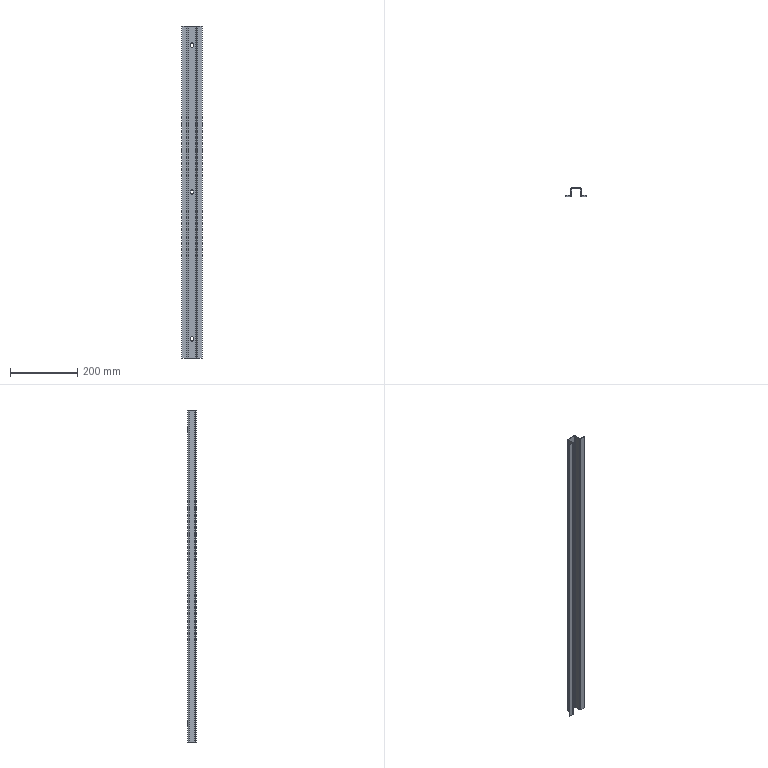Part | STEP file | SYL_0392D6J1SYL0380DJ100-399186 | 1 solid | 56 faces | box 60 x 25 x 984 mm | volume 197947 mm3 | plane 36 | cylinder 20 | commonest cylinder face diameters 7 x12 4 x4 8 x4
STEP:
#1=CARTESIAN_POINT('',(-3.5,23.,-431.5));
#2=VERTEX_POINT('',#1);
#3=CARTESIAN_POINT('',(-3.5,25.,-431.5));
#4=VERTEX_POINT('',#3);
#5=CARTESIAN_POINT('',(-3.5,25.,-431.5));
#6=DIRECTION('',(0.,1.,0.));
#7=VECTOR('',#6,1000.);
#8=LINE('',#5,#7);
#9=EDGE_CURVE('',#2,#4,#8,.T.);
#10=ORIENTED_EDGE('',*,*,#9,.F.);
#11=CARTESIAN_POINT('',(-3.5,23.,-438.5));
#12=VERTEX_POINT('',#11);
#13=CARTESIAN_POINT('',(-3.5,23.,-492.));
#14=DIRECTION('',(0.,0.,1.));
#15=VECTOR('',#14,1000.);
#16=LINE('',#13,#15);
#17=EDGE_CURVE('',#12,#2,#16,.T.);
#18=ORIENTED_EDGE('',*,*,#17,.F.);
#19=CARTESIAN_POINT('',(-3.5,25.,-438.5));
#20=VERTEX_POINT('',#19);
#21=CARTESIAN_POINT('',(-3.5,25.,-438.5));
#22=DIRECTION('',(0.,1.,0.));
#23=VECTOR('',#22,1000.);
#24=LINE('',#21,#23);
#25=EDGE_CURVE('',#12,#20,#24,.T.);
#26=ORIENTED_EDGE('',*,*,#25,.T.);
#27=CARTESIAN_POINT('',(-3.5,25.,-438.5));
#28=DIRECTION('',(0.,0.,1.));
#29=VECTOR('',#28,1000.);
#30=LINE('',#27,#29);
#31=EDGE_CURVE('',#20,#4,#30,.T.);
#32=ORIENTED_EDGE('',*,*,#31,.T.);
#33=EDGE_LOOP('',(#10,#18,#26,#32));
#34=FACE_OUTER_BOUND('',#33,.T.);
#35=CARTESIAN_POINT('',(-3.5,25.,-438.5));
#36=DIRECTION('',(1.,0.,0.));
#37=DIRECTION('',(0.,0.,1.));
#38=AXIS2_PLACEMENT_3D('',#35,#36,#37);
#39=PLANE('',#38);
#40=ADVANCED_FACE('',(#34),#39,.T.);
#41=ORIENTED_EDGE('',*,*,#25,.F.);
#42=CARTESIAN_POINT('',(0.,23.,-442.));
#43=VERTEX_POINT('',#42);
#44=CARTESIAN_POINT('',(0.,23.,-438.5));
#45=DIRECTION('',(0.,-1.,0.));
#46=DIRECTION('',(0.,0.,-1.));
#47=AXIS2_PLACEMENT_3D('',#44,#45,#46);
#48=CIRCLE('',#47,3.5);
#49=EDGE_CURVE('',#12,#43,#48,.T.);
#50=ORIENTED_EDGE('',*,*,#49,.T.);
#51=CARTESIAN_POINT('',(0.,25.,-442.));
#52=VERTEX_POINT('',#51);
#53=CARTESIAN_POINT('',(0.,25.,-442.));
#54=DIRECTION('',(0.,1.,0.));
#55=VECTOR('',#54,1000.);
#56=LINE('',#53,#55);
#57=EDGE_CURVE('',#43,#52,#56,.T.);
#58=ORIENTED_EDGE('',*,*,#57,.T.);
#59=CARTESIAN_POINT('',(0.,25.,-438.5));
#60=DIRECTION('',(0.,-1.,0.));
#61=DIRECTION('',(-1.,0.,0.));
#62=AXIS2_PLACEMENT_3D('',#59,#60,#61);
#63=CIRCLE('',#62,3.5);
#64=EDGE_CURVE('',#20,#52,#63,.T.);
#65=ORIENTED_EDGE('',*,*,#64,.F.);
#66=EDGE_LOOP('',(#41,#50,#58,#65));
#67=FACE_OUTER_BOUND('',#66,.T.);
#68=CARTESIAN_POINT('',(0.,25.,-438.5));
#69=DIRECTION('',(0.,-1.,0.));
#70=DIRECTION('',(0.,0.,-1.));
#71=AXIS2_PLACEMENT_3D('',#68,#69,#70);
#72=CYLINDRICAL_SURFACE('',#71,3.5);
#73=ADVANCED_FACE('',(#67),#72,.F.);
#74=ORIENTED_EDGE('',*,*,#57,.F.);
#75=CARTESIAN_POINT('',(3.5,23.,-438.5));
#76=VERTEX_POINT('',#75);
#77=CARTESIAN_POINT('',(0.,23.,-438.5));
#78=DIRECTION('',(0.,-1.,0.));
#79=DIRECTION('',(0.,0.,-1.));
#80=AXIS2_PLACEMENT_3D('',#77,#78,#79);
#81=CIRCLE('',#80,3.5);
#82=EDGE_CURVE('',#43,#76,#81,.T.);
#83=ORIENTED_EDGE('',*,*,#82,.T.);
#84=CARTESIAN_POINT('',(3.5,25.,-438.5));
#85=VERTEX_POINT('',#84);
#86=CARTESIAN_POINT('',(3.5,25.,-438.5));
#87=DIRECTION('',(0.,1.,0.));
#88=VECTOR('',#87,1000.);
#89=LINE('',#86,#88);
#90=EDGE_CURVE('',#76,#85,#89,.T.);
#91=ORIENTED_EDGE('',*,*,#90,.T.);
#92=CARTESIAN_POINT('',(0.,25.,-438.5));
#93=DIRECTION('',(0.,-1.,0.));
#94=DIRECTION('',(0.,0.,-1.));
#95=AXIS2_PLACEMENT_3D('',#92,#93,#94);
#96=CIRCLE('',#95,3.5);
#97=EDGE_CURVE('',#52,#85,#96,.T.);
#98=ORIENTED_EDGE('',*,*,#97,.F.);
#99=EDGE_LOOP('',(#74,#83,#91,#98));
#100=FACE_OUTER_BOUND('',#99,.T.);
#101=CARTESIAN_POINT('',(0.,25.,-438.5));
#102=DIRECTION('',(0.,-1.,0.));
#103=DIRECTION('',(0.,0.,-1.));
#104=AXIS2_PLACEMENT_3D('',#101,#102,#103);
#105=CYLINDRICAL_SURFACE('',#104,3.5);
#106=ADVANCED_FACE('',(#100),#105,.F.);
#107=ORIENTED_EDGE('',*,*,#90,.F.);
#108=CARTESIAN_POINT('',(3.5,23.,-431.5));
#109=VERTEX_POINT('',#108);
#110=CARTESIAN_POINT('',(3.5,23.,-492.));
#111=DIRECTION('',(0.,0.,-1.));
#112=VECTOR('',#111,1000.);
#113=LINE('',#110,#112);
#114=EDGE_CURVE('',#109,#76,#113,.T.);
#115=ORIENTED_EDGE('',*,*,#114,.F.);
#116=CARTESIAN_POINT('',(3.5,25.,-431.5));
#117=VERTEX_POINT('',#116);
#118=CARTESIAN_POINT('',(3.5,25.,-431.5));
#119=DIRECTION('',(0.,1.,0.));
#120=VECTOR('',#119,1000.);
#121=LINE('',#118,#120);
#122=EDGE_CURVE('',#109,#117,#121,.T.);
#123=ORIENTED_EDGE('',*,*,#122,.T.);
#124=CARTESIAN_POINT('',(3.5,25.,-431.5));
#125=DIRECTION('',(0.,0.,-1.));
#126=VECTOR('',#125,1000.);
#127=LINE('',#124,#126);
#128=EDGE_CURVE('',#117,#85,#127,.T.);
#129=ORIENTED_EDGE('',*,*,#128,.T.);
#130=EDGE_LOOP('',(#107,#115,#123,#129));
#131=FACE_OUTER_BOUND('',#130,.T.);
#132=CARTESIAN_POINT('',(3.5,25.,-431.5));
#133=DIRECTION('',(-1.,0.,0.));
#134=DIRECTION('',(0.,0.,-1.));
#135=AXIS2_PLACEMENT_3D('',#132,#133,#134);
#136=PLANE('',#135);
#137=ADVANCED_FACE('',(#131),#136,.T.);
#138=ORIENTED_EDGE('',*,*,#122,.F.);
#139=CARTESIAN_POINT('',(0.,23.,-428.));
#140=VERTEX_POINT('',#139);
#141=CARTESIAN_POINT('',(0.,23.,-431.5));
#142=DIRECTION('',(0.,-1.,0.));
#143=DIRECTION('',(0.,0.,-1.));
#144=AXIS2_PLACEMENT_3D('',#141,#142,#143);
#145=CIRCLE('',#144,3.5);
#146=EDGE_CURVE('',#109,#140,#145,.T.);
#147=ORIENTED_EDGE('',*,*,#146,.T.);
#148=CARTESIAN_POINT('',(0.,25.,-428.));
#149=VERTEX_POINT('',#148);
#150=CARTESIAN_POINT('',(0.,25.,-428.));
#151=DIRECTION('',(0.,1.,0.));
#152=VECTOR('',#151,1000.);
#153=LINE('',#150,#152);
#154=EDGE_CURVE('',#140,#149,#153,.T.);
#155=ORIENTED_EDGE('',*,*,#154,.T.);
#156=CARTESIAN_POINT('',(0.,25.,-431.5));
#157=DIRECTION('',(0.,-1.,0.));
#158=DIRECTION('',(1.,0.,0.));
#159=AXIS2_PLACEMENT_3D('',#156,#157,#158);
#160=CIRCLE('',#159,3.5);
#161=EDGE_CURVE('',#117,#149,#160,.T.);
#162=ORIENTED_EDGE('',*,*,#161,.F.);
#163=EDGE_LOOP('',(#138,#147,#155,#162));
#164=FACE_OUTER_BOUND('',#163,.T.);
#165=CARTESIAN_POINT('',(0.,25.,-431.5));
#166=DIRECTION('',(0.,-1.,0.));
#167=DIRECTION('',(0.,0.,-1.));
#168=AXIS2_PLACEMENT_3D('',#165,#166,#167);
#169=CYLINDRICAL_SURFACE('',#168,3.5);
#170=ADVANCED_FACE('',(#164),#169,.F.);
#171=CARTESIAN_POINT('',(-3.5,23.,3.5));
#172=VERTEX_POINT('',#171);
#173=CARTESIAN_POINT('',(-3.5,25.,3.5));
#174=VERTEX_POINT('',#173);
#175=CARTESIAN_POINT('',(-3.5,25.,3.5));
#176=DIRECTION('',(0.,1.,0.));
#177=VECTOR('',#176,1000.);
#178=LINE('',#175,#177);
#179=EDGE_CURVE('',#172,#174,#178,.T.);
#180=ORIENTED_EDGE('',*,*,#179,.F.);
#181=CARTESIAN_POINT('',(-3.5,23.,-3.5));
#182=VERTEX_POINT('',#181);
#183=CARTESIAN_POINT('',(-3.5,23.,-492.));
#184=DIRECTION('',(0.,0.,1.));
#185=VECTOR('',#184,1000.);
#186=LINE('',#183,#185);
#187=EDGE_CURVE('',#182,#172,#186,.T.);
#188=ORIENTED_EDGE('',*,*,#187,.F.);
#189=CARTESIAN_POINT('',(-3.5,25.,-3.5));
#190=VERTEX_POINT('',#189);
#191=CARTESIAN_POINT('',(-3.5,25.,-3.5));
#192=DIRECTION('',(0.,1.,0.));
#193=VECTOR('',#192,1000.);
#194=LINE('',#191,#193);
#195=EDGE_CURVE('',#182,#190,#194,.T.);
#196=ORIENTED_EDGE('',*,*,#195,.T.);
#197=CARTESIAN_POINT('',(-3.5,25.,-3.5));
#198=DIRECTION('',(0.,0.,1.));
#199=VECTOR('',#198,1000.);
#200=LINE('',#197,#199);
#201=EDGE_CURVE('',#190,#174,#200,.T.);
#202=ORIENTED_EDGE('',*,*,#201,.T.);
#203=EDGE_LOOP('',(#180,#188,#196,#202));
#204=FACE_OUTER_BOUND('',#203,.T.);
#205=CARTESIAN_POINT('',(-3.5,25.,-3.5));
#206=DIRECTION('',(1.,0.,0.));
#207=DIRECTION('',(0.,0.,1.));
#208=AXIS2_PLACEMENT_3D('',#205,#206,#207);
#209=PLANE('',#208);
#210=ADVANCED_FACE('',(#204),#209,.T.);
#211=ORIENTED_EDGE('',*,*,#195,.F.);
#212=CARTESIAN_POINT('',(0.,23.,-7.));
#213=VERTEX_POINT('',#212);
#214=CARTESIAN_POINT('',(0.,23.,-3.5));
#215=DIRECTION('',(0.,-1.,0.));
#216=DIRECTION('',(0.,0.,-1.));
#217=AXIS2_PLACEMENT_3D('',#214,#215,#216);
#218=CIRCLE('',#217,3.5);
#219=EDGE_CURVE('',#182,#213,#218,.T.);
#220=ORIENTED_EDGE('',*,*,#219,.T.);
#221=CARTESIAN_POINT('',(0.,25.,-7.));
#222=VERTEX_POINT('',#221);
#223=CARTESIAN_POINT('',(0.,25.,-7.));
#224=DIRECTION('',(0.,1.,0.));
#225=VECTOR('',#224,1000.);
#226=LINE('',#223,#225);
#227=EDGE_CURVE('',#213,#222,#226,.T.);
#228=ORIENTED_EDGE('',*,*,#227,.T.);
#229=CARTESIAN_POINT('',(0.,25.,-3.5));
#230=DIRECTION('',(0.,-1.,0.));
#231=DIRECTION('',(-1.,0.,0.));
#232=AXIS2_PLACEMENT_3D('',#229,#230,#231);
#233=CIRCLE('',#232,3.5);
#234=EDGE_CURVE('',#190,#222,#233,.T.);
#235=ORIENTED_EDGE('',*,*,#234,.F.);
#236=EDGE_LOOP('',(#211,#220,#228,#235));
#237=FACE_OUTER_BOUND('',#236,.T.);
#238=CARTESIAN_POINT('',(0.,25.,-3.5));
#239=DIRECTION('',(0.,-1.,0.));
#240=DIRECTION('',(0.,0.,-1.));
#241=AXIS2_PLACEMENT_3D('',#238,#239,#240);
#242=CYLINDRICAL_SURFACE('',#241,3.5);
#243=ADVANCED_FACE('',(#237),#242,.F.);
#244=ORIENTED_EDGE('',*,*,#227,.F.);
#245=CARTESIAN_POINT('',(3.5,23.,-3.5));
#246=VERTEX_POINT('',#245);
#247=CARTESIAN_POINT('',(0.,23.,-3.5));
#248=DIRECTION('',(0.,-1.,0.));
#249=DIRECTION('',(0.,0.,-1.));
#250=AXIS2_PLACEMENT_3D('',#247,#248,#249);
#251=CIRCLE('',#250,3.5);
#252=EDGE_CURVE('',#213,#246,#251,.T.);
#253=ORIENTED_EDGE('',*,*,#252,.T.);
#254=CARTESIAN_POINT('',(3.5,25.,-3.5));
#255=VERTEX_POINT('',#254);
#256=CARTESIAN_POINT('',(3.5,25.,-3.5));
#257=DIRECTION('',(0.,1.,0.));
#258=VECTOR('',#257,1000.);
#259=LINE('',#256,#258);
#260=EDGE_CURVE('',#246,#255,#259,.T.);
#261=ORIENTED_EDGE('',*,*,#260,.T.);
#262=CARTESIAN_POINT('',(0.,25.,-3.5));
#263=DIRECTION('',(0.,-1.,0.));
#264=DIRECTION('',(0.,0.,-1.));
#265=AXIS2_PLACEMENT_3D('',#262,#263,#264);
#266=CIRCLE('',#265,3.5);
#267=EDGE_CURVE('',#222,#255,#266,.T.);
#268=ORIENTED_EDGE('',*,*,#267,.F.);
#269=EDGE_LOOP('',(#244,#253,#261,#268));
#270=FACE_OUTER_BOUND('',#269,.T.);
#271=CARTESIAN_POINT('',(0.,25.,-3.5));
#272=DIRECTION('',(0.,-1.,0.));
#273=DIRECTION('',(0.,0.,-1.));
#274=AXIS2_PLACEMENT_3D('',#271,#272,#273);
#275=CYLINDRICAL_SURFACE('',#274,3.5);
#276=ADVANCED_FACE('',(#270),#275,.F.);
#277=ORIENTED_EDGE('',*,*,#260,.F.);
#278=CARTESIAN_POINT('',(3.5,23.,3.5));
#279=VERTEX_POINT('',#278);
#280=CARTESIAN_POINT('',(3.5,23.,-492.));
#281=DIRECTION('',(0.,0.,-1.));
#282=VECTOR('',#281,1000.);
#283=LINE('',#280,#282);
#284=EDGE_CURVE('',#279,#246,#283,.T.);
#285=ORIENTED_EDGE('',*,*,#284,.F.);
#286=CARTESIAN_POINT('',(3.5,25.,3.5));
#287=VERTEX_POINT('',#286);
#288=CARTESIAN_POINT('',(3.5,25.,3.5));
#289=DIRECTION('',(0.,1.,0.));
#290=VECTOR('',#289,1000.);
#291=LINE('',#288,#290);
#292=EDGE_CURVE('',#279,#287,#291,.T.);
#293=ORIENTED_EDGE('',*,*,#292,.T.);
#294=CARTESIAN_POINT('',(3.5,25.,3.5));
#295=DIRECTION('',(0.,0.,-1.));
#296=VECTOR('',#295,1000.);
#297=LINE('',#294,#296);
#298=EDGE_CURVE('',#287,#255,#297,.T.);
#299=ORIENTED_EDGE('',*,*,#298,.T.);
#300=EDGE_LOOP('',(#277,#285,#293,#299));
#301=FACE_OUTER_BOUND('',#300,.T.);
#302=CARTESIAN_POINT('',(3.5,25.,3.5));
#303=DIRECTION('',(-1.,0.,0.));
#304=DIRECTION('',(0.,0.,-1.));
#305=AXIS2_PLACEMENT_3D('',#302,#303,#304);
#306=PLANE('',#305);
#307=ADVANCED_FACE('',(#301),#306,.T.);
#308=ORIENTED_EDGE('',*,*,#292,.F.);
#309=CARTESIAN_POINT('',(0.,23.,7.));
#310=VERTEX_POINT('',#309);
#311=CARTESIAN_POINT('',(0.,23.,3.5));
#312=DIRECTION('',(0.,-1.,0.));
#313=DIRECTION('',(0.,0.,-1.));
#314=AXIS2_PLACEMENT_3D('',#311,#312,#313);
#315=CIRCLE('',#314,3.5);
#316=EDGE_CURVE('',#279,#310,#315,.T.);
#317=ORIENTED_EDGE('',*,*,#316,.T.);
#318=CARTESIAN_POINT('',(0.,25.,7.));
#319=VERTEX_POINT('',#318);
#320=CARTESIAN_POINT('',(0.,25.,7.));
#321=DIRECTION('',(0.,1.,0.));
#322=VECTOR('',#321,1000.);
#323=LINE('',#320,#322);
#324=EDGE_CURVE('',#310,#319,#323,.T.);
#325=ORIENTED_EDGE('',*,*,#324,.T.);
#326=CARTESIAN_POINT('',(0.,25.,3.5));
#327=DIRECTION('',(0.,-1.,0.));
#328=DIRECTION('',(1.,0.,0.));
#329=AXIS2_PLACEMENT_3D('',#326,#327,#328);
#330=CIRCLE('',#329,3.5);
#331=EDGE_CURVE('',#287,#319,#330,.T.);
#332=ORIENTED_EDGE('',*,*,#331,.F.);
#333=EDGE_LOOP('',(#308,#317,#325,#332));
#334=FACE_OUTER_BOUND('',#333,.T.);
#335=CARTESIAN_POINT('',(0.,25.,3.5));
#336=DIRECTION('',(0.,-1.,0.));
#337=DIRECTION('',(0.,0.,-1.));
#338=AXIS2_PLACEMENT_3D('',#335,#336,#337);
#339=CYLINDRICAL_SURFACE('',#338,3.5);
#340=ADVANCED_FACE('',(#334),#339,.F.);
#341=CARTESIAN_POINT('',(-3.5,23.,438.5));
#342=VERTEX_POINT('',#341);
#343=CARTESIAN_POINT('',(-3.5,25.,438.5));
#344=VERTEX_POINT('',#343);
#345=CARTESIAN_POINT('',(-3.5,25.,438.5));
#346=DIRECTION('',(0.,1.,0.));
#347=VECTOR('',#346,1000.);
#348=LINE('',#345,#347);
#349=EDGE_CURVE('',#342,#344,#348,.T.);
#350=ORIENTED_EDGE('',*,*,#349,.F.);
#351=CARTESIAN_POINT('',(-3.5,23.,431.5));
#352=VERTEX_POINT('',#351);
#353=CARTESIAN_POINT('',(-3.5,23.,-492.));
#354=DIRECTION('',(0.,0.,1.));
#355=VECTOR('',#354,1000.);
#356=LINE('',#353,#355);
#357=EDGE_CURVE('',#352,#342,#356,.T.);
#358=ORIENTED_EDGE('',*,*,#357,.F.);
#359=CARTESIAN_POINT('',(-3.5,25.,431.5));
#360=VERTEX_POINT('',#359);
#361=CARTESIAN_POINT('',(-3.5,25.,431.5));
#362=DIRECTION('',(0.,1.,0.));
#363=VECTOR('',#362,1000.);
#364=LINE('',#361,#363);
#365=EDGE_CURVE('',#352,#360,#364,.T.);
#366=ORIENTED_EDGE('',*,*,#365,.T.);
#367=CARTESIAN_POINT('',(-3.5,25.,431.5));
#368=DIRECTION('',(0.,0.,1.));
#369=VECTOR('',#368,1000.);
#370=LINE('',#367,#369);
#371=EDGE_CURVE('',#360,#344,#370,.T.);
#372=ORIENTED_EDGE('',*,*,#371,.T.);
#373=EDGE_LOOP('',(#350,#358,#366,#372));
#374=FACE_OUTER_BOUND('',#373,.T.);
#375=CARTESIAN_POINT('',(-3.5,25.,431.5));
#376=DIRECTION('',(1.,0.,0.));
#377=DIRECTION('',(0.,0.,1.));
#378=AXIS2_PLACEMENT_3D('',#375,#376,#377);
#379=PLANE('',#378);
#380=ADVANCED_FACE('',(#374),#379,.T.);
#381=ORIENTED_EDGE('',*,*,#365,.F.);
#382=CARTESIAN_POINT('',(0.,23.,428.));
#383=VERTEX_POINT('',#382);
#384=CARTESIAN_POINT('',(0.,23.,431.5));
#385=DIRECTION('',(0.,-1.,0.));
#386=DIRECTION('',(0.,0.,-1.));
#387=AXIS2_PLACEMENT_3D('',#384,#385,#386);
#388=CIRCLE('',#387,3.5);
#389=EDGE_CURVE('',#352,#383,#388,.T.);
#390=ORIENTED_EDGE('',*,*,#389,.T.);
#391=CARTESIAN_POINT('',(0.,25.,428.));
#392=VERTEX_POINT('',#391);
#393=CARTESIAN_POINT('',(0.,25.,428.));
#394=DIRECTION('',(0.,1.,0.));
#395=VECTOR('',#394,1000.);
#396=LINE('',#393,#395);
#397=EDGE_CURVE('',#383,#392,#396,.T.);
#398=ORIENTED_EDGE('',*,*,#397,.T.);
#399=CARTESIAN_POINT('',(0.,25.,431.5));
#400=DIRECTION('',(0.,-1.,0.));
#401=DIRECTION('',(-1.,0.,0.));
#402=AXIS2_PLACEMENT_3D('',#399,#400,#401);
#403=CIRCLE('',#402,3.5);
#404=EDGE_CURVE('',#360,#392,#403,.T.);
#405=ORIENTED_EDGE('',*,*,#404,.F.);
#406=EDGE_LOOP('',(#381,#390,#398,#405));
#407=FACE_OUTER_BOUND('',#406,.T.);
#408=CARTESIAN_POINT('',(0.,25.,431.5));
#409=DIRECTION('',(0.,-1.,0.));
#410=DIRECTION('',(0.,0.,-1.));
#411=AXIS2_PLACEMENT_3D('',#408,#409,#410);
#412=CYLINDRICAL_SURFACE('',#411,3.5);
#413=ADVANCED_FACE('',(#407),#412,.F.);
#414=ORIENTED_EDGE('',*,*,#397,.F.);
#415=CARTESIAN_POINT('',(3.5,23.,431.5));
#416=VERTEX_POINT('',#415);
#417=CARTESIAN_POINT('',(0.,23.,431.5));
#418=DIRECTION('',(0.,-1.,0.));
#419=DIRECTION('',(0.,0.,-1.));
#420=AXIS2_PLACEMENT_3D('',#417,#418,#419);
#421=CIRCLE('',#420,3.5);
#422=EDGE_CURVE('',#383,#416,#421,.T.);
#423=ORIENTED_EDGE('',*,*,#422,.T.);
#424=CARTESIAN_POINT('',(3.5,25.,431.5));
#425=VERTEX_POINT('',#424);
#426=CARTESIAN_POINT('',(3.5,25.,431.5));
#427=DIRECTION('',(0.,1.,0.));
#428=VECTOR('',#427,1000.);
#429=LINE('',#426,#428);
#430=EDGE_CURVE('',#416,#425,#429,.T.);
#431=ORIENTED_EDGE('',*,*,#430,.T.);
#432=CARTESIAN_POINT('',(0.,25.,431.5));
#433=DIRECTION('',(0.,-1.,0.));
#434=DIRECTION('',(0.,0.,-1.));
#435=AXIS2_PLACEMENT_3D('',#432,#433,#434);
#436=CIRCLE('',#435,3.5);
#437=EDGE_CURVE('',#392,#425,#436,.T.);
#438=ORIENTED_EDGE('',*,*,#437,.F.);
#439=EDGE_LOOP('',(#414,#423,#431,#438));
#440=FACE_OUTER_BOUND('',#439,.T.);
#441=CARTESIAN_POINT('',(0.,25.,431.5));
#442=DIRECTION('',(0.,-1.,0.));
#443=DIRECTION('',(0.,0.,-1.));
#444=AXIS2_PLACEMENT_3D('',#441,#442,#443);
#445=CYLINDRICAL_SURFACE('',#444,3.5);
#446=ADVANCED_FACE('',(#440),#445,.F.);
#447=ORIENTED_EDGE('',*,*,#430,.F.);
#448=CARTESIAN_POINT('',(3.5,23.,438.5));
#449=VERTEX_POINT('',#448);
#450=CARTESIAN_POINT('',(3.5,23.,-492.));
#451=DIRECTION('',(0.,0.,-1.));
#452=VECTOR('',#451,1000.);
#453=LINE('',#450,#452);
#454=EDGE_CURVE('',#449,#416,#453,.T.);
#455=ORIENTED_EDGE('',*,*,#454,.F.);
#456=CARTESIAN_POINT('',(3.5,25.,438.5));
#457=VERTEX_POINT('',#456);
#458=CARTESIAN_POINT('',(3.5,25.,438.5));
#459=DIRECTION('',(0.,1.,0.));
#460=VECTOR('',#459,1000.);
#461=LINE('',#458,#460);
#462=EDGE_CURVE('',#449,#457,#461,.T.);
#463=ORIENTED_EDGE('',*,*,#462,.T.);
#464=CARTESIAN_POINT('',(3.5,25.,438.5));
#465=DIRECTION('',(0.,0.,-1.));
#466=VECTOR('',#465,1000.);
#467=LINE('',#464,#466);
#468=EDGE_CURVE('',#457,#425,#467,.T.);
#469=ORIENTED_EDGE('',*,*,#468,.T.);
#470=EDGE_LOOP('',(#447,#455,#463,#469));
#471=FACE_OUTER_BOUND('',#470,.T.);
#472=CARTESIAN_POINT('',(3.5,25.,438.5));
#473=DIRECTION('',(-1.,0.,0.));
#474=DIRECTION('',(0.,0.,-1.));
#475=AXIS2_PLACEMENT_3D('',#472,#473,#474);
#476=PLANE('',#475);
#477=ADVANCED_FACE('',(#471),#476,.T.);
#478=ORIENTED_EDGE('',*,*,#462,.F.);
#479=CARTESIAN_POINT('',(0.,23.,442.));
#480=VERTEX_POINT('',#479);
#481=CARTESIAN_POINT('',(0.,23.,438.5));
#482=DIRECTION('',(0.,-1.,0.));
#483=DIRECTION('',(0.,0.,-1.));
#484=AXIS2_PLACEMENT_3D('',#481,#482,#483);
#485=CIRCLE('',#484,3.5);
#486=EDGE_CURVE('',#449,#480,#485,.T.);
#487=ORIENTED_EDGE('',*,*,#486,.T.);
#488=CARTESIAN_POINT('',(0.,25.,442.));
#489=VERTEX_POINT('',#488);
#490=CARTESIAN_POINT('',(0.,25.,442.));
#491=DIRECTION('',(0.,1.,0.));
#492=VECTOR('',#491,1000.);
#493=LINE('',#490,#492);
#494=EDGE_CURVE('',#480,#489,#493,.T.);
#495=ORIENTED_EDGE('',*,*,#494,.T.);
#496=CARTESIAN_POINT('',(0.,25.,438.5));
#497=DIRECTION('',(0.,-1.,0.));
#498=DIRECTION('',(1.,0.,0.));
#499=AXIS2_PLACEMENT_3D('',#496,#497,#498);
#500=CIRCLE('',#499,3.5);
#501=EDGE_CURVE('',#457,#489,#500,.T.);
#502=ORIENTED_EDGE('',*,*,#501,.F.);
#503=EDGE_LOOP('',(#478,#487,#495,#502));
#504=FACE_OUTER_BOUND('',#503,.T.);
#505=CARTESIAN_POINT('',(0.,25.,438.5));
#506=DIRECTION('',(0.,-1.,0.));
#507=DIRECTION('',(0.,0.,-1.));
#508=AXIS2_PLACEMENT_3D('',#505,#506,#507);
#509=CYLINDRICAL_SURFACE('',#508,3.5);
#510=ADVANCED_FACE('',(#504),#509,.F.);
#511=CARTESIAN_POINT('',(-30.,0.,-492.));
#512=VERTEX_POINT('',#511);
#513=CARTESIAN_POINT('',(-30.,2.,-492.));
#514=VERTEX_POINT('',#513);
#515=CARTESIAN_POINT('',(-30.,2.,-492.));
#516=DIRECTION('',(0.,1.,0.));
#517=VECTOR('',#516,1000.);
#518=LINE('',#515,#517);
#519=EDGE_CURVE('',#512,#514,#518,.T.);
#520=ORIENTED_EDGE('',*,*,#519,.F.);
#521=CARTESIAN_POINT('',(-30.,0.,492.));
#522=VERTEX_POINT('',#521);
#523=CARTESIAN_POINT('',(-30.,0.,-492.));
#524=DIRECTION('',(0.,0.,-1.));
#525=VECTOR('',#524,1000.);
#526=LINE('',#523,#525);
#527=EDGE_CURVE('',#522,#512,#526,.T.);
#528=ORIENTED_EDGE('',*,*,#527,.F.);
#529=CARTESIAN_POINT('',(-30.,2.,492.));
#530=VERTEX_POINT('',#529);
#531=CARTESIAN_POINT('',(-30.,2.,492.));
#532=DIRECTION('',(0.,1.,0.));
#533=VECTOR('',#532,1000.);
#534=LINE('',#531,#533);
#535=EDGE_CURVE('',#522,#530,#534,.T.);
#536=ORIENTED_EDGE('',*,*,#535,.T.);
#537=CARTESIAN_POINT('',(-30.,2.,492.));
#538=DIRECTION('',(0.,0.,-1.));
#539=VECTOR('',#538,1000.);
#540=LINE('',#537,#539);
#541=EDGE_CURVE('',#530,#514,#540,.T.);
#542=ORIENTED_EDGE('',*,*,#541,.T.);
#543=EDGE_LOOP('',(#520,#528,#536,#542));
#544=FACE_OUTER_BOUND('',#543,.T.);
#545=CARTESIAN_POINT('',(-30.,2.,492.));
#546=DIRECTION('',(-1.,0.,0.));
#547=DIRECTION('',(0.,0.,-1.));
#548=AXIS2_PLACEMENT_3D('',#545,#546,#547);
#549=PLANE('',#548);
#550=ADVANCED_FACE('',(#544),#549,.T.);
#551=ORIENTED_EDGE('',*,*,#535,.F.);
#552=CARTESIAN_POINT('',(-17.,0.,492.));
#553=VERTEX_POINT('',#552);
#554=CARTESIAN_POINT('',(-30.,0.,492.));
#555=DIRECTION('',(-1.,0.,0.));
#556=VECTOR('',#555,1000.);
#557=LINE('',#554,#556);
#558=EDGE_CURVE('',#553,#522,#557,.T.);
#559=ORIENTED_EDGE('',*,*,#558,.F.);
#560=CARTESIAN_POINT('',(-17.,2.,492.));
#561=VERTEX_POINT('',#560);
#562=CARTESIAN_POINT('',(-17.,2.,492.));
#563=DIRECTION('',(0.,1.,0.));
#564=VECTOR('',#563,1000.);
#565=LINE('',#562,#564);
#566=EDGE_CURVE('',#553,#561,#565,.T.);
#567=ORIENTED_EDGE('',*,*,#566,.T.);
#568=CARTESIAN_POINT('',(-17.,2.,492.));
#569=DIRECTION('',(-1.,0.,0.));
#570=VECTOR('',#569,1000.);
#571=LINE('',#568,#570);
#572=EDGE_CURVE('',#561,#530,#571,.T.);
#573=ORIENTED_EDGE('',*,*,#572,.T.);
#574=EDGE_LOOP('',(#551,#559,#567,#573));
#575=FACE_OUTER_BOUND('',#574,.T.);
#576=CARTESIAN_POINT('',(-17.,2.,492.));
#577=DIRECTION('',(0.,0.,1.));
#578=DIRECTION('',(-1.,0.,0.));
#579=AXIS2_PLACEMENT_3D('',#576,#577,#578);
#580=PLANE('',#579);
#581=ADVANCED_FACE('',(#575),#580,.T.);
#582=ORIENTED_EDGE('',*,*,#566,.F.);
#583=CARTESIAN_POINT('',(-13.,4.,492.));
#584=VERTEX_POINT('',#583);
#585=CARTESIAN_POINT('',(-17.,4.,492.));
#586=DIRECTION('',(0.,0.,-1.));
#587=DIRECTION('',(1.,0.,0.));
#588=AXIS2_PLACEMENT_3D('',#585,#586,#587);
#589=CIRCLE('',#588,4.);
#590=EDGE_CURVE('',#584,#553,#589,.T.);
#591=ORIENTED_EDGE('',*,*,#590,.F.);
#592=CARTESIAN_POINT('',(-15.,4.,492.));
#593=VERTEX_POINT('',#592);
#594=CARTESIAN_POINT('',(-15.,4.,492.));
#595=DIRECTION('',(-1.,0.,0.));
#596=VECTOR('',#595,1000.);
#597=LINE('',#594,#596);
#598=EDGE_CURVE('',#584,#593,#597,.T.);
#599=ORIENTED_EDGE('',*,*,#598,.T.);
#600=CARTESIAN_POINT('',(-17.,4.,492.));
#601=DIRECTION('',(0.,0.,-1.));
#602=DIRECTION('',(1.,0.,0.));
#603=AXIS2_PLACEMENT_3D('',#600,#601,#602);
#604=CIRCLE('',#603,2.);
#605=EDGE_CURVE('',#593,#561,#604,.T.);
#606=ORIENTED_EDGE('',*,*,#605,.T.);
#607=EDGE_LOOP('',(#582,#591,#599,#606));
#608=FACE_OUTER_BOUND('',#607,.T.);
#609=CARTESIAN_POINT('',(-17.,4.,492.));
#610=DIRECTION('',(0.,0.,1.));
#611=DIRECTION('',(1.,0.,0.));
#612=AXIS2_PLACEMENT_3D('',#609,#610,#611);
#613=PLANE('',#612);
#614=ADVANCED_FACE('',(#608),#613,.T.);
#615=ORIENTED_EDGE('',*,*,#598,.F.);
#616=CARTESIAN_POINT('',(-13.,21.,492.));
#617=VERTEX_POINT('',#616);
#618=CARTESIAN_POINT('',(-13.,4.,492.));
#619=DIRECTION('',(0.,-1.,0.));
#620=VECTOR('',#619,1000.);
#621=LINE('',#618,#620);
#622=EDGE_CURVE('',#617,#584,#621,.T.);
#623=ORIENTED_EDGE('',*,*,#622,.F.);
#624=CARTESIAN_POINT('',(-15.,21.,492.));
#625=VERTEX_POINT('',#624);
#626=CARTESIAN_POINT('',(-15.,21.,492.));
#627=DIRECTION('',(-1.,0.,0.));
#628=VECTOR('',#627,1000.);
#629=LINE('',#626,#628);
#630=EDGE_CURVE('',#617,#625,#629,.T.);
#631=ORIENTED_EDGE('',*,*,#630,.T.);
#632=CARTESIAN_POINT('',(-15.,21.,492.));
#633=DIRECTION('',(0.,-1.,0.));
#634=VECTOR('',#633,1000.);
#635=LINE('',#632,#634);
#636=EDGE_CURVE('',#625,#593,#635,.T.);
#637=ORIENTED_EDGE('',*,*,#636,.T.);
#638=EDGE_LOOP('',(#615,#623,#631,#637));
#639=FACE_OUTER_BOUND('',#638,.T.);
#640=CARTESIAN_POINT('',(-15.,21.,492.));
#641=DIRECTION('',(0.,0.,1.));
#642=DIRECTION('',(0.,-1.,0.));
#643=AXIS2_PLACEMENT_3D('',#640,#641,#642);
#644=PLANE('',#643);
#645=ADVANCED_FACE('',(#639),#644,.T.);
#646=ORIENTED_EDGE('',*,*,#630,.F.);
#647=CARTESIAN_POINT('',(-11.,23.,492.));
#648=VERTEX_POINT('',#647);
#649=CARTESIAN_POINT('',(-11.,21.,492.));
#650=DIRECTION('',(0.,0.,1.));
#651=DIRECTION('',(1.,0.,0.));
#652=AXIS2_PLACEMENT_3D('',#649,#650,#651);
#653=CIRCLE('',#652,2.);
#654=EDGE_CURVE('',#648,#617,#653,.T.);
#655=ORIENTED_EDGE('',*,*,#654,.F.);
#656=CARTESIAN_POINT('',(-11.,25.,492.));
#657=VERTEX_POINT('',#656);
#658=CARTESIAN_POINT('',(-11.,25.,492.));
#659=DIRECTION('',(0.,1.,0.));
#660=VECTOR('',#659,1000.);
#661=LINE('',#658,#660);
#662=EDGE_CURVE('',#648,#657,#661,.T.);
#663=ORIENTED_EDGE('',*,*,#662,.T.);
#664=CARTESIAN_POINT('',(-11.,21.,492.));
#665=DIRECTION('',(0.,0.,1.));
#666=DIRECTION('',(0.,1.,0.));
#667=AXIS2_PLACEMENT_3D('',#664,#665,#666);
#668=CIRCLE('',#667,4.);
#669=EDGE_CURVE('',#657,#625,#668,.T.);
#670=ORIENTED_EDGE('',*,*,#669,.T.);
#671=EDGE_LOOP('',(#646,#655,#663,#670));
#672=FACE_OUTER_BOUND('',#671,.T.);
#673=CARTESIAN_POINT('',(-11.,21.,492.));
#674=DIRECTION('',(0.,0.,-1.));
#675=DIRECTION('',(-1.,0.,0.));
#676=AXIS2_PLACEMENT_3D('',#673,#674,#675);
#677=PLANE('',#676);
#678=ADVANCED_FACE('',(#672),#677,.F.);
#679=ORIENTED_EDGE('',*,*,#662,.F.);
#680=CARTESIAN_POINT('',(11.,23.,492.));
#681=VERTEX_POINT('',#680);
#682=CARTESIAN_POINT('',(-11.,23.,492.));
#683=DIRECTION('',(-1.,0.,0.));
#684=VECTOR('',#683,1000.);
#685=LINE('',#682,#684);
#686=EDGE_CURVE('',#681,#648,#685,.T.);
#687=ORIENTED_EDGE('',*,*,#686,.F.);
#688=CARTESIAN_POINT('',(11.,25.,492.));
#689=VERTEX_POINT('',#688);
#690=CARTESIAN_POINT('',(11.,25.,492.));
#691=DIRECTION('',(0.,1.,0.));
#692=VECTOR('',#691,1000.);
#693=LINE('',#690,#692);
#694=EDGE_CURVE('',#681,#689,#693,.T.);
#695=ORIENTED_EDGE('',*,*,#694,.T.);
#696=CARTESIAN_POINT('',(11.,25.,492.));
#697=DIRECTION('',(-1.,0.,0.));
#698=VECTOR('',#697,1000.);
#699=LINE('',#696,#698);
#700=EDGE_CURVE('',#689,#657,#699,.T.);
#701=ORIENTED_EDGE('',*,*,#700,.T.);
#702=EDGE_LOOP('',(#679,#687,#695,#701));
#703=FACE_OUTER_BOUND('',#702,.T.);
#704=CARTESIAN_POINT('',(11.,25.,492.));
#705=DIRECTION('',(0.,0.,1.));
#706=DIRECTION('',(-1.,0.,0.));
#707=AXIS2_PLACEMENT_3D('',#704,#705,#706);
#708=PLANE('',#707);
#709=ADVANCED_FACE('',(#703),#708,.T.);
#710=ORIENTED_EDGE('',*,*,#694,.F.);
#711=CARTESIAN_POINT('',(13.,21.,492.));
#712=VERTEX_POINT('',#711);
#713=CARTESIAN_POINT('',(11.,21.,492.));
#714=DIRECTION('',(0.,0.,1.));
#715=DIRECTION('',(1.,0.,0.));
#716=AXIS2_PLACEMENT_3D('',#713,#714,#715);
#717=CIRCLE('',#716,2.);
#718=EDGE_CURVE('',#712,#681,#717,.T.);
#719=ORIENTED_EDGE('',*,*,#718,.F.);
#720=CARTESIAN_POINT('',(15.,21.,492.));
#721=VERTEX_POINT('',#720);
#722=CARTESIAN_POINT('',(15.,21.,492.));
#723=DIRECTION('',(1.,0.,0.));
#724=VECTOR('',#723,1000.);
#725=LINE('',#722,#724);
#726=EDGE_CURVE('',#712,#721,#725,.T.);
#727=ORIENTED_EDGE('',*,*,#726,.T.);
#728=CARTESIAN_POINT('',(11.,21.,492.));
#729=DIRECTION('',(0.,0.,1.));
#730=DIRECTION('',(1.,0.,0.));
#731=AXIS2_PLACEMENT_3D('',#728,#729,#730);
#732=CIRCLE('',#731,4.);
#733=EDGE_CURVE('',#721,#689,#732,.T.);
#734=ORIENTED_EDGE('',*,*,#733,.T.);
#735=EDGE_LOOP('',(#710,#719,#727,#734));
#736=FACE_OUTER_BOUND('',#735,.T.);
#737=CARTESIAN_POINT('',(11.,21.,492.));
#738=DIRECTION('',(0.,0.,-1.));
#739=DIRECTION('',(-1.,0.,0.));
#740=AXIS2_PLACEMENT_3D('',#737,#738,#739);
#741=PLANE('',#740);
#742=ADVANCED_FACE('',(#736),#741,.F.);
#743=ORIENTED_EDGE('',*,*,#726,.F.);
#744=CARTESIAN_POINT('',(13.,4.,492.));
#745=VERTEX_POINT('',#744);
#746=CARTESIAN_POINT('',(13.,21.,492.));
#747=DIRECTION('',(0.,1.,0.));
#748=VECTOR('',#747,1000.);
#749=LINE('',#746,#748);
#750=EDGE_CURVE('',#745,#712,#749,.T.);
#751=ORIENTED_EDGE('',*,*,#750,.F.);
#752=CARTESIAN_POINT('',(15.,4.,492.));
#753=VERTEX_POINT('',#752);
#754=CARTESIAN_POINT('',(15.,4.,492.));
#755=DIRECTION('',(1.,0.,0.));
#756=VECTOR('',#755,1000.);
#757=LINE('',#754,#756);
#758=EDGE_CURVE('',#745,#753,#757,.T.);
#759=ORIENTED_EDGE('',*,*,#758,.T.);
#760=CARTESIAN_POINT('',(15.,4.,492.));
#761=DIRECTION('',(0.,1.,0.));
#762=VECTOR('',#761,1000.);
#763=LINE('',#760,#762);
#764=EDGE_CURVE('',#753,#721,#763,.T.);
#765=ORIENTED_EDGE('',*,*,#764,.T.);
#766=EDGE_LOOP('',(#743,#751,#759,#765));
#767=FACE_OUTER_BOUND('',#766,.T.);
#768=CARTESIAN_POINT('',(15.,4.,492.));
#769=DIRECTION('',(0.,0.,1.));
#770=DIRECTION('',(0.,1.,0.));
#771=AXIS2_PLACEMENT_3D('',#768,#769,#770);
#772=PLANE('',#771);
#773=ADVANCED_FACE('',(#767),#772,.T.);
#774=ORIENTED_EDGE('',*,*,#758,.F.);
#775=CARTESIAN_POINT('',(17.,0.,492.));
#776=VERTEX_POINT('',#775);
#777=CARTESIAN_POINT('',(17.,4.,492.));
#778=DIRECTION('',(0.,0.,-1.));
#779=DIRECTION('',(1.,0.,0.));
#780=AXIS2_PLACEMENT_3D('',#777,#778,#779);
#781=CIRCLE('',#780,4.);
#782=EDGE_CURVE('',#776,#745,#781,.T.);
#783=ORIENTED_EDGE('',*,*,#782,.F.);
#784=CARTESIAN_POINT('',(17.,2.,492.));
#785=VERTEX_POINT('',#784);
#786=CARTESIAN_POINT('',(17.,2.,492.));
#787=DIRECTION('',(0.,1.,0.));
#788=VECTOR('',#787,1000.);
#789=LINE('',#786,#788);
#790=EDGE_CURVE('',#776,#785,#789,.T.);
#791=ORIENTED_EDGE('',*,*,#790,.T.);
#792=CARTESIAN_POINT('',(17.,4.,492.));
#793=DIRECTION('',(0.,0.,-1.));
#794=DIRECTION('',(0.,-1.,0.));
#795=AXIS2_PLACEMENT_3D('',#792,#793,#794);
#796=CIRCLE('',#795,2.);
#797=EDGE_CURVE('',#785,#753,#796,.T.);
#798=ORIENTED_EDGE('',*,*,#797,.T.);
#799=EDGE_LOOP('',(#774,#783,#791,#798));
#800=FACE_OUTER_BOUND('',#799,.T.);
#801=CARTESIAN_POINT('',(17.,4.,492.));
#802=DIRECTION('',(0.,0.,1.));
#803=DIRECTION('',(1.,0.,0.));
#804=AXIS2_PLACEMENT_3D('',#801,#802,#803);
#805=PLANE('',#804);
#806=ADVANCED_FACE('',(#800),#805,.T.);
#807=ORIENTED_EDGE('',*,*,#790,.F.);
#808=CARTESIAN_POINT('',(30.,0.,492.));
#809=VERTEX_POINT('',#808);
#810=CARTESIAN_POINT('',(17.,0.,492.));
#811=DIRECTION('',(-1.,0.,0.));
#812=VECTOR('',#811,1000.);
#813=LINE('',#810,#812);
#814=EDGE_CURVE('',#809,#776,#813,.T.);
#815=ORIENTED_EDGE('',*,*,#814,.F.);
#816=CARTESIAN_POINT('',(30.,2.,492.));
#817=VERTEX_POINT('',#816);
#818=CARTESIAN_POINT('',(30.,2.,492.));
#819=DIRECTION('',(0.,1.,0.));
#820=VECTOR('',#819,1000.);
#821=LINE('',#818,#820);
#822=EDGE_CURVE('',#809,#817,#821,.T.);
#823=ORIENTED_EDGE('',*,*,#822,.T.);
#824=CARTESIAN_POINT('',(30.,2.,492.));
#825=DIRECTION('',(-1.,0.,0.));
#826=VECTOR('',#825,1000.);
#827=LINE('',#824,#826);
#828=EDGE_CURVE('',#817,#785,#827,.T.);
#829=ORIENTED_EDGE('',*,*,#828,.T.);
#830=EDGE_LOOP('',(#807,#815,#823,#829));
#831=FACE_OUTER_BOUND('',#830,.T.);
#832=CARTESIAN_POINT('',(30.,2.,492.));
#833=DIRECTION('',(0.,0.,1.));
#834=DIRECTION('',(-1.,0.,0.));
#835=AXIS2_PLACEMENT_3D('',#832,#833,#834);
#836=PLANE('',#835);
#837=ADVANCED_FACE('',(#831),#836,.T.);
#838=ORIENTED_EDGE('',*,*,#822,.F.);
#839=CARTESIAN_POINT('',(30.,0.,-492.));
#840=VERTEX_POINT('',#839);
#841=CARTESIAN_POINT('',(30.,0.,-492.));
#842=DIRECTION('',(0.,0.,-1.));
#843=VECTOR('',#842,1000.);
#844=LINE('',#841,#843);
#845=EDGE_CURVE('',#809,#840,#844,.T.);
#846=ORIENTED_EDGE('',*,*,#845,.T.);
#847=CARTESIAN_POINT('',(30.,2.,-492.));
#848=VERTEX_POINT('',#847);
#849=CARTESIAN_POINT('',(30.,2.,-492.));
#850=DIRECTION('',(0.,1.,0.));
#851=VECTOR('',#850,1000.);
#852=LINE('',#849,#851);
#853=EDGE_CURVE('',#840,#848,#852,.T.);
#854=ORIENTED_EDGE('',*,*,#853,.T.);
#855=CARTESIAN_POINT('',(30.,2.,492.));
#856=DIRECTION('',(0.,0.,-1.));
#857=VECTOR('',#856,1000.);
#858=LINE('',#855,#857);
#859=EDGE_CURVE('',#817,#848,#858,.T.);
#860=ORIENTED_EDGE('',*,*,#859,.F.);
#861=EDGE_LOOP('',(#838,#846,#854,#860));
#862=FACE_OUTER_BOUND('',#861,.T.);
#863=CARTESIAN_POINT('',(30.,2.,492.));
#864=DIRECTION('',(-1.,0.,0.));
#865=DIRECTION('',(0.,0.,-1.));
#866=AXIS2_PLACEMENT_3D('',#863,#864,#865);
#867=PLANE('',#866);
#868=ADVANCED_FACE('',(#862),#867,.F.);
#869=ORIENTED_EDGE('',*,*,#853,.F.);
#870=CARTESIAN_POINT('',(17.,0.,-492.));
#871=VERTEX_POINT('',#870);
#872=CARTESIAN_POINT('',(17.,0.,-492.));
#873=DIRECTION('',(-1.,0.,0.));
#874=VECTOR('',#873,1000.);
#875=LINE('',#872,#874);
#876=EDGE_CURVE('',#840,#871,#875,.T.);
#877=ORIENTED_EDGE('',*,*,#876,.T.);
#878=CARTESIAN_POINT('',(17.,2.,-492.));
#879=VERTEX_POINT('',#878);
#880=CARTESIAN_POINT('',(17.,2.,-492.));
#881=DIRECTION('',(0.,1.,0.));
#882=VECTOR('',#881,1000.);
#883=LINE('',#880,#882);
#884=EDGE_CURVE('',#871,#879,#883,.T.);
#885=ORIENTED_EDGE('',*,*,#884,.T.);
#886=CARTESIAN_POINT('',(30.,2.,-492.));
#887=DIRECTION('',(-1.,0.,0.));
#888=VECTOR('',#887,1000.);
#889=LINE('',#886,#888);
#890=EDGE_CURVE('',#848,#879,#889,.T.);
#891=ORIENTED_EDGE('',*,*,#890,.F.);
#892=EDGE_LOOP('',(#869,#877,#885,#891));
#893=FACE_OUTER_BOUND('',#892,.T.);
#894=CARTESIAN_POINT('',(30.,2.,-492.));
#895=DIRECTION('',(0.,0.,1.));
#896=DIRECTION('',(-1.,0.,0.));
#897=AXIS2_PLACEMENT_3D('',#894,#895,#896);
#898=PLANE('',#897);
#899=ADVANCED_FACE('',(#893),#898,.F.);
#900=ORIENTED_EDGE('',*,*,#884,.F.);
#901=CARTESIAN_POINT('',(13.,4.,-492.));
#902=VERTEX_POINT('',#901);
#903=CARTESIAN_POINT('',(17.,4.,-492.));
#904=DIRECTION('',(0.,0.,1.));
#905=DIRECTION('',(1.,0.,0.));
#906=AXIS2_PLACEMENT_3D('',#903,#904,#905);
#907=CIRCLE('',#906,4.);
#908=EDGE_CURVE('',#902,#871,#907,.T.);
#909=ORIENTED_EDGE('',*,*,#908,.F.);
#910=CARTESIAN_POINT('',(15.,4.,-492.));
#911=VERTEX_POINT('',#910);
#912=CARTESIAN_POINT('',(15.,4.,-492.));
#913=DIRECTION('',(1.,0.,0.));
#914=VECTOR('',#913,1000.);
#915=LINE('',#912,#914);
#916=EDGE_CURVE('',#902,#911,#915,.T.);
#917=ORIENTED_EDGE('',*,*,#916,.T.);
#918=CARTESIAN_POINT('',(17.,4.,-492.));
#919=DIRECTION('',(0.,0.,1.));
#920=DIRECTION('',(-1.,0.,0.));
#921=AXIS2_PLACEMENT_3D('',#918,#919,#920);
#922=CIRCLE('',#921,2.);
#923=EDGE_CURVE('',#911,#879,#922,.T.);
#924=ORIENTED_EDGE('',*,*,#923,.T.);
#925=EDGE_LOOP('',(#900,#909,#917,#924));
#926=FACE_OUTER_BOUND('',#925,.T.);
#927=CARTESIAN_POINT('',(17.,4.,-492.));
#928=DIRECTION('',(0.,0.,-1.));
#929=DIRECTION('',(-1.,0.,0.));
#930=AXIS2_PLACEMENT_3D('',#927,#928,#929);
#931=PLANE('',#930);
#932=ADVANCED_FACE('',(#926),#931,.T.);
#933=ORIENTED_EDGE('',*,*,#916,.F.);
#934=CARTESIAN_POINT('',(13.,21.,-492.));
#935=VERTEX_POINT('',#934);
#936=CARTESIAN_POINT('',(13.,21.,-492.));
#937=DIRECTION('',(0.,1.,0.));
#938=VECTOR('',#937,1000.);
#939=LINE('',#936,#938);
#940=EDGE_CURVE('',#902,#935,#939,.T.);
#941=ORIENTED_EDGE('',*,*,#940,.T.);
#942=CARTESIAN_POINT('',(15.,21.,-492.));
#943=VERTEX_POINT('',#942);
#944=CARTESIAN_POINT('',(15.,21.,-492.));
#945=DIRECTION('',(1.,0.,0.));
#946=VECTOR('',#945,1000.);
#947=LINE('',#944,#946);
#948=EDGE_CURVE('',#935,#943,#947,.T.);
#949=ORIENTED_EDGE('',*,*,#948,.T.);
#950=CARTESIAN_POINT('',(15.,4.,-492.));
#951=DIRECTION('',(0.,1.,0.));
#952=VECTOR('',#951,1000.);
#953=LINE('',#950,#952);
#954=EDGE_CURVE('',#911,#943,#953,.T.);
#955=ORIENTED_EDGE('',*,*,#954,.F.);
#956=EDGE_LOOP('',(#933,#941,#949,#955));
#957=FACE_OUTER_BOUND('',#956,.T.);
#958=CARTESIAN_POINT('',(15.,4.,-492.));
#959=DIRECTION('',(0.,0.,1.));
#960=DIRECTION('',(0.,1.,0.));
#961=AXIS2_PLACEMENT_3D('',#958,#959,#960);
#962=PLANE('',#961);
#963=ADVANCED_FACE('',(#957),#962,.F.);
#964=ORIENTED_EDGE('',*,*,#948,.F.);
#965=CARTESIAN_POINT('',(11.,23.,-492.));
#966=VERTEX_POINT('',#965);
#967=CARTESIAN_POINT('',(11.,21.,-492.));
#968=DIRECTION('',(0.,0.,-1.));
#969=DIRECTION('',(1.,0.,0.));
#970=AXIS2_PLACEMENT_3D('',#967,#968,#969);
#971=CIRCLE('',#970,2.);
#972=EDGE_CURVE('',#966,#935,#971,.T.);
#973=ORIENTED_EDGE('',*,*,#972,.F.);
#974=CARTESIAN_POINT('',(11.,25.,-492.));
#975=VERTEX_POINT('',#974);
#976=CARTESIAN_POINT('',(11.,25.,-492.));
#977=DIRECTION('',(0.,1.,0.));
#978=VECTOR('',#977,1000.);
#979=LINE('',#976,#978);
#980=EDGE_CURVE('',#966,#975,#979,.T.);
#981=ORIENTED_EDGE('',*,*,#980,.T.);
#982=CARTESIAN_POINT('',(11.,21.,-492.));
#983=DIRECTION('',(0.,0.,-1.));
#984=DIRECTION('',(0.,1.,0.));
#985=AXIS2_PLACEMENT_3D('',#982,#983,#984);
#986=CIRCLE('',#985,4.);
#987=EDGE_CURVE('',#975,#943,#986,.T.);
#988=ORIENTED_EDGE('',*,*,#987,.T.);
#989=EDGE_LOOP('',(#964,#973,#981,#988));
#990=FACE_OUTER_BOUND('',#989,.T.);
#991=CARTESIAN_POINT('',(11.,21.,-492.));
#992=DIRECTION('',(0.,0.,1.));
#993=DIRECTION('',(1.,0.,0.));
#994=AXIS2_PLACEMENT_3D('',#991,#992,#993);
#995=PLANE('',#994);
#996=ADVANCED_FACE('',(#990),#995,.F.);
#997=ORIENTED_EDGE('',*,*,#980,.F.);
#998=CARTESIAN_POINT('',(-11.,23.,-492.));
#999=VERTEX_POINT('',#998);
#1000=CARTESIAN_POINT('',(-11.,23.,-492.));
#1001=DIRECTION('',(-1.,0.,0.));
#1002=VECTOR('',#1001,1000.);
#1003=LINE('',#1000,#1002);
#1004=EDGE_CURVE('',#966,#999,#1003,.T.);
#1005=ORIENTED_EDGE('',*,*,#1004,.T.);
#1006=CARTESIAN_POINT('',(-11.,25.,-492.));
#1007=VERTEX_POINT('',#1006);
#1008=CARTESIAN_POINT('',(-11.,25.,-492.));
#1009=DIRECTION('',(0.,1.,0.));
#1010=VECTOR('',#1009,1000.);
#1011=LINE('',#1008,#1010);
#1012=EDGE_CURVE('',#999,#1007,#1011,.T.);
#1013=ORIENTED_EDGE('',*,*,#1012,.T.);
#1014=CARTESIAN_POINT('',(11.,25.,-492.));
#1015=DIRECTION('',(-1.,0.,0.));
#1016=VECTOR('',#1015,1000.);
#1017=LINE('',#1014,#1016);
#1018=EDGE_CURVE('',#975,#1007,#1017,.T.);
#1019=ORIENTED_EDGE('',*,*,#1018,.F.);
#1020=EDGE_LOOP('',(#997,#1005,#1013,#1019));
#1021=FACE_OUTER_BOUND('',#1020,.T.);
#1022=CARTESIAN_POINT('',(11.,25.,-492.));
#1023=DIRECTION('',(0.,0.,1.));
#1024=DIRECTION('',(-1.,0.,0.));
#1025=AXIS2_PLACEMENT_3D('',#1022,#1023,#1024);
#1026=PLANE('',#1025);
#1027=ADVANCED_FACE('',(#1021),#1026,.F.);
#1028=ORIENTED_EDGE('',*,*,#1012,.F.);
#1029=CARTESIAN_POINT('',(-13.,21.,-492.));
#1030=VERTEX_POINT('',#1029);
#1031=CARTESIAN_POINT('',(-11.,21.,-492.));
#1032=DIRECTION('',(0.,0.,-1.));
#1033=DIRECTION('',(1.,0.,0.));
#1034=AXIS2_PLACEMENT_3D('',#1031,#1032,#1033);
#1035=CIRCLE('',#1034,2.);
#1036=EDGE_CURVE('',#1030,#999,#1035,.T.);
#1037=ORIENTED_EDGE('',*,*,#1036,.F.);
#1038=CARTESIAN_POINT('',(-15.,21.,-492.));
#1039=VERTEX_POINT('',#1038);
#1040=CARTESIAN_POINT('',(-15.,21.,-492.));
#1041=DIRECTION('',(-1.,0.,0.));
#1042=VECTOR('',#1041,1000.);
#1043=LINE('',#1040,#1042);
#1044=EDGE_CURVE('',#1030,#1039,#1043,.T.);
#1045=ORIENTED_EDGE('',*,*,#1044,.T.);
#1046=CARTESIAN_POINT('',(-11.,21.,-492.));
#1047=DIRECTION('',(0.,0.,-1.));
#1048=DIRECTION('',(-1.,0.,0.));
#1049=AXIS2_PLACEMENT_3D('',#1046,#1047,#1048);
#1050=CIRCLE('',#1049,4.);
#1051=EDGE_CURVE('',#1039,#1007,#1050,.T.);
#1052=ORIENTED_EDGE('',*,*,#1051,.T.);
#1053=EDGE_LOOP('',(#1028,#1037,#1045,#1052));
#1054=FACE_OUTER_BOUND('',#1053,.T.);
#1055=CARTESIAN_POINT('',(-11.,21.,-492.));
#1056=DIRECTION('',(0.,0.,1.));
#1057=DIRECTION('',(1.,0.,0.));
#1058=AXIS2_PLACEMENT_3D('',#1055,#1056,#1057);
#1059=PLANE('',#1058);
#1060=ADVANCED_FACE('',(#1054),#1059,.F.);
#1061=ORIENTED_EDGE('',*,*,#1044,.F.);
#1062=CARTESIAN_POINT('',(-13.,4.,-492.));
#1063=VERTEX_POINT('',#1062);
#1064=CARTESIAN_POINT('',(-13.,4.,-492.));
#1065=DIRECTION('',(0.,-1.,0.));
#1066=VECTOR('',#1065,1000.);
#1067=LINE('',#1064,#1066);
#1068=EDGE_CURVE('',#1030,#1063,#1067,.T.);
#1069=ORIENTED_EDGE('',*,*,#1068,.T.);
#1070=CARTESIAN_POINT('',(-15.,4.,-492.));
#1071=VERTEX_POINT('',#1070);
#1072=CARTESIAN_POINT('',(-15.,4.,-492.));
#1073=DIRECTION('',(-1.,0.,0.));
#1074=VECTOR('',#1073,1000.);
#1075=LINE('',#1072,#1074);
#1076=EDGE_CURVE('',#1063,#1071,#1075,.T.);
#1077=ORIENTED_EDGE('',*,*,#1076,.T.);
#1078=CARTESIAN_POINT('',(-15.,21.,-492.));
#1079=DIRECTION('',(0.,-1.,0.));
#1080=VECTOR('',#1079,1000.);
#1081=LINE('',#1078,#1080);
#1082=EDGE_CURVE('',#1039,#1071,#1081,.T.);
#1083=ORIENTED_EDGE('',*,*,#1082,.F.);
#1084=EDGE_LOOP('',(#1061,#1069,#1077,#1083));
#1085=FACE_OUTER_BOUND('',#1084,.T.);
#1086=CARTESIAN_POINT('',(-15.,21.,-492.));
#1087=DIRECTION('',(0.,0.,1.));
#1088=DIRECTION('',(0.,-1.,0.));
#1089=AXIS2_PLACEMENT_3D('',#1086,#1087,#1088);
#1090=PLANE('',#1089);
#1091=ADVANCED_FACE('',(#1085),#1090,.F.);
#1092=ORIENTED_EDGE('',*,*,#1076,.F.);
#1093=CARTESIAN_POINT('',(-17.,0.,-492.));
#1094=VERTEX_POINT('',#1093);
#1095=CARTESIAN_POINT('',(-17.,4.,-492.));
#1096=DIRECTION('',(0.,0.,1.));
#1097=DIRECTION('',(1.,0.,0.));
#1098=AXIS2_PLACEMENT_3D('',#1095,#1096,#1097);
#1099=CIRCLE('',#1098,4.);
#1100=EDGE_CURVE('',#1094,#1063,#1099,.T.);
#1101=ORIENTED_EDGE('',*,*,#1100,.F.);
#1102=CARTESIAN_POINT('',(-17.,2.,-492.));
#1103=VERTEX_POINT('',#1102);
#1104=CARTESIAN_POINT('',(-17.,2.,-492.));
#1105=DIRECTION('',(0.,1.,0.));
#1106=VECTOR('',#1105,1000.);
#1107=LINE('',#1104,#1106);
#1108=EDGE_CURVE('',#1094,#1103,#1107,.T.);
#1109=ORIENTED_EDGE('',*,*,#1108,.T.);
#1110=CARTESIAN_POINT('',(-17.,4.,-492.));
#1111=DIRECTION('',(0.,0.,1.));
#1112=DIRECTION('',(0.,-1.,0.));
#1113=AXIS2_PLACEMENT_3D('',#1110,#1111,#1112);
#1114=CIRCLE('',#1113,2.);
#1115=EDGE_CURVE('',#1103,#1071,#1114,.T.);
#1116=ORIENTED_EDGE('',*,*,#1115,.T.);
#1117=EDGE_LOOP('',(#1092,#1101,#1109,#1116));
#1118=FACE_OUTER_BOUND('',#1117,.T.);
#1119=CARTESIAN_POINT('',(-17.,4.,-492.));
#1120=DIRECTION('',(0.,0.,-1.));
#1121=DIRECTION('',(-1.,0.,0.));
#1122=AXIS2_PLACEMENT_3D('',#1119,#1120,#1121);
#1123=PLANE('',#1122);
#1124=ADVANCED_FACE('',(#1118),#1123,.T.);
#1125=CARTESIAN_POINT('',(0.,23.,438.5));
#1126=DIRECTION('',(0.,-1.,0.));
#1127=DIRECTION('',(0.,0.,-1.));
#1128=AXIS2_PLACEMENT_3D('',#1125,#1126,#1127);
#1129=CIRCLE('',#1128,3.5);
#1130=EDGE_CURVE('',#480,#342,#1129,.T.);
#1131=ORIENTED_EDGE('',*,*,#1130,.T.);
#1132=ORIENTED_EDGE('',*,*,#349,.T.);
#1133=CARTESIAN_POINT('',(0.,25.,438.5));
#1134=DIRECTION('',(0.,-1.,0.));
#1135=DIRECTION('',(0.,0.,1.));
#1136=AXIS2_PLACEMENT_3D('',#1133,#1134,#1135);
#1137=CIRCLE('',#1136,3.5);
#1138=EDGE_CURVE('',#489,#344,#1137,.T.);
#1139=ORIENTED_EDGE('',*,*,#1138,.F.);
#1140=ORIENTED_EDGE('',*,*,#494,.F.);
#1141=EDGE_LOOP('',(#1131,#1132,#1139,#1140));
#1142=FACE_OUTER_BOUND('',#1141,.T.);
#1143=CARTESIAN_POINT('',(0.,25.,438.5));
#1144=DIRECTION('',(0.,-1.,0.));
#1145=DIRECTION('',(0.,0.,-1.));
#1146=AXIS2_PLACEMENT_3D('',#1143,#1144,#1145);
#1147=CYLINDRICAL_SURFACE('',#1146,3.5);
#1148=ADVANCED_FACE('',(#1142),#1147,.F.);
#1149=CARTESIAN_POINT('',(0.,23.,3.5));
#1150=DIRECTION('',(0.,-1.,0.));
#1151=DIRECTION('',(0.,0.,-1.));
#1152=AXIS2_PLACEMENT_3D('',#1149,#1150,#1151);
#1153=CIRCLE('',#1152,3.5);
#1154=EDGE_CURVE('',#310,#172,#1153,.T.);
#1155=ORIENTED_EDGE('',*,*,#1154,.T.);
#1156=ORIENTED_EDGE('',*,*,#179,.T.);
#1157=CARTESIAN_POINT('',(0.,25.,3.5));
#1158=DIRECTION('',(0.,-1.,0.));
#1159=DIRECTION('',(0.,0.,1.));
#1160=AXIS2_PLACEMENT_3D('',#1157,#1158,#1159);
#1161=CIRCLE('',#1160,3.5);
#1162=EDGE_CURVE('',#319,#174,#1161,.T.);
#1163=ORIENTED_EDGE('',*,*,#1162,.F.);
#1164=ORIENTED_EDGE('',*,*,#324,.F.);
#1165=EDGE_LOOP('',(#1155,#1156,#1163,#1164));
#1166=FACE_OUTER_BOUND('',#1165,.T.);
#1167=CARTESIAN_POINT('',(0.,25.,3.5));
#1168=DIRECTION('',(0.,-1.,0.));
#1169=DIRECTION('',(0.,0.,-1.));
#1170=AXIS2_PLACEMENT_3D('',#1167,#1168,#1169);
#1171=CYLINDRICAL_SURFACE('',#1170,3.5);
#1172=ADVANCED_FACE('',(#1166),#1171,.F.);
#1173=CARTESIAN_POINT('',(0.,23.,-431.5));
#1174=DIRECTION('',(0.,-1.,0.));
#1175=DIRECTION('',(0.,0.,-1.));
#1176=AXIS2_PLACEMENT_3D('',#1173,#1174,#1175);
#1177=CIRCLE('',#1176,3.5);
#1178=EDGE_CURVE('',#140,#2,#1177,.T.);
#1179=ORIENTED_EDGE('',*,*,#1178,.T.);
#1180=ORIENTED_EDGE('',*,*,#9,.T.);
#1181=CARTESIAN_POINT('',(0.,25.,-431.5));
#1182=DIRECTION('',(0.,-1.,0.));
#1183=DIRECTION('',(0.,0.,1.));
#1184=AXIS2_PLACEMENT_3D('',#1181,#1182,#1183);
#1185=CIRCLE('',#1184,3.5);
#1186=EDGE_CURVE('',#149,#4,#1185,.T.);
#1187=ORIENTED_EDGE('',*,*,#1186,.F.);
#1188=ORIENTED_EDGE('',*,*,#154,.F.);
#1189=EDGE_LOOP('',(#1179,#1180,#1187,#1188));
#1190=FACE_OUTER_BOUND('',#1189,.T.);
#1191=CARTESIAN_POINT('',(0.,25.,-431.5));
#1192=DIRECTION('',(0.,-1.,0.));
#1193=DIRECTION('',(0.,0.,-1.));
#1194=AXIS2_PLACEMENT_3D('',#1191,#1192,#1193);
#1195=CYLINDRICAL_SURFACE('',#1194,3.5);
#1196=ADVANCED_FACE('',(#1190),#1195,.F.);
#1197=CARTESIAN_POINT('',(-30.,0.,-492.));
#1198=DIRECTION('',(-1.,0.,0.));
#1199=VECTOR('',#1198,1000.);
#1200=LINE('',#1197,#1199);
#1201=EDGE_CURVE('',#1094,#512,#1200,.T.);
#1202=ORIENTED_EDGE('',*,*,#1201,.T.);
#1203=ORIENTED_EDGE('',*,*,#519,.T.);
#1204=CARTESIAN_POINT('',(-17.,2.,-492.));
#1205=DIRECTION('',(-1.,0.,0.));
#1206=VECTOR('',#1205,1000.);
#1207=LINE('',#1204,#1206);
#1208=EDGE_CURVE('',#1103,#514,#1207,.T.);
#1209=ORIENTED_EDGE('',*,*,#1208,.F.);
#1210=ORIENTED_EDGE('',*,*,#1108,.F.);
#1211=EDGE_LOOP('',(#1202,#1203,#1209,#1210));
#1212=FACE_OUTER_BOUND('',#1211,.T.);
#1213=CARTESIAN_POINT('',(-17.,2.,-492.));
#1214=DIRECTION('',(0.,0.,1.));
#1215=DIRECTION('',(-1.,0.,0.));
#1216=AXIS2_PLACEMENT_3D('',#1213,#1214,#1215);
#1217=PLANE('',#1216);
#1218=ADVANCED_FACE('',(#1212),#1217,.F.);
#1219=CARTESIAN_POINT('',(-15.,4.,492.));
#1220=DIRECTION('',(0.,0.,-1.));
#1221=VECTOR('',#1220,1000.);
#1222=LINE('',#1219,#1221);
#1223=EDGE_CURVE('',#593,#1071,#1222,.T.);
#1224=ORIENTED_EDGE('',*,*,#1223,.T.);
#1225=ORIENTED_EDGE('',*,*,#1115,.F.);
#1226=CARTESIAN_POINT('',(-17.,2.,-492.));
#1227=DIRECTION('',(0.,0.,1.));
#1228=VECTOR('',#1227,1000.);
#1229=LINE('',#1226,#1228);
#1230=EDGE_CURVE('',#1103,#561,#1229,.T.);
#1231=ORIENTED_EDGE('',*,*,#1230,.T.);
#1232=ORIENTED_EDGE('',*,*,#605,.F.);
#1233=EDGE_LOOP('',(#1224,#1225,#1231,#1232));
#1234=FACE_OUTER_BOUND('',#1233,.T.);
#1235=CARTESIAN_POINT('',(-17.,4.,-492.));
#1236=DIRECTION('',(0.,0.,1.));
#1237=DIRECTION('',(1.,0.,0.));
#1238=AXIS2_PLACEMENT_3D('',#1235,#1236,#1237);
#1239=CYLINDRICAL_SURFACE('',#1238,2.);
#1240=ADVANCED_FACE('',(#1234),#1239,.F.);
#1241=ORIENTED_EDGE('',*,*,#1230,.F.);
#1242=ORIENTED_EDGE('',*,*,#1208,.T.);
#1243=ORIENTED_EDGE('',*,*,#541,.F.);
#1244=ORIENTED_EDGE('',*,*,#572,.F.);
#1245=EDGE_LOOP('',(#1241,#1242,#1243,#1244));
#1246=FACE_OUTER_BOUND('',#1245,.T.);
#1247=CARTESIAN_POINT('',(-30.,2.,-492.));
#1248=DIRECTION('',(0.,-1.,0.));
#1249=DIRECTION('',(0.,0.,-1.));
#1250=AXIS2_PLACEMENT_3D('',#1247,#1248,#1249);
#1251=PLANE('',#1250);
#1252=ADVANCED_FACE('',(#1246),#1251,.F.);
#1253=ORIENTED_EDGE('',*,*,#1051,.F.);
#1254=CARTESIAN_POINT('',(-15.,21.,-492.));
#1255=DIRECTION('',(0.,0.,1.));
#1256=VECTOR('',#1255,1000.);
#1257=LINE('',#1254,#1256);
#1258=EDGE_CURVE('',#1039,#625,#1257,.T.);
#1259=ORIENTED_EDGE('',*,*,#1258,.T.);
#1260=ORIENTED_EDGE('',*,*,#669,.F.);
#1261=CARTESIAN_POINT('',(-11.,25.,492.));
#1262=DIRECTION('',(0.,0.,-1.));
#1263=VECTOR('',#1262,1000.);
#1264=LINE('',#1261,#1263);
#1265=EDGE_CURVE('',#657,#1007,#1264,.T.);
#1266=ORIENTED_EDGE('',*,*,#1265,.T.);
#1267=EDGE_LOOP('',(#1253,#1259,#1260,#1266));
#1268=FACE_OUTER_BOUND('',#1267,.T.);
#1269=CARTESIAN_POINT('',(-11.,21.,-492.));
#1270=DIRECTION('',(0.,0.,1.));
#1271=DIRECTION('',(1.,0.,0.));
#1272=AXIS2_PLACEMENT_3D('',#1269,#1270,#1271);
#1273=CYLINDRICAL_SURFACE('',#1272,4.);
#1274=ADVANCED_FACE('',(#1268),#1273,.T.);
#1275=ORIENTED_EDGE('',*,*,#1258,.F.);
#1276=ORIENTED_EDGE('',*,*,#1082,.T.);
#1277=ORIENTED_EDGE('',*,*,#1223,.F.);
#1278=ORIENTED_EDGE('',*,*,#636,.F.);
#1279=EDGE_LOOP('',(#1275,#1276,#1277,#1278));
#1280=FACE_OUTER_BOUND('',#1279,.T.);
#1281=CARTESIAN_POINT('',(-15.,4.,-492.));
#1282=DIRECTION('',(1.,0.,0.));
#1283=DIRECTION('',(0.,1.,0.));
#1284=AXIS2_PLACEMENT_3D('',#1281,#1282,#1283);
#1285=PLANE('',#1284);
#1286=ADVANCED_FACE('',(#1280),#1285,.F.);
#1287=ORIENTED_EDGE('',*,*,#987,.F.);
#1288=CARTESIAN_POINT('',(11.,25.,-492.));
#1289=DIRECTION('',(0.,0.,1.));
#1290=VECTOR('',#1289,1000.);
#1291=LINE('',#1288,#1290);
#1292=EDGE_CURVE('',#975,#689,#1291,.T.);
#1293=ORIENTED_EDGE('',*,*,#1292,.T.);
#1294=ORIENTED_EDGE('',*,*,#733,.F.);
#1295=CARTESIAN_POINT('',(15.,21.,492.));
#1296=DIRECTION('',(0.,0.,-1.));
#1297=VECTOR('',#1296,1000.);
#1298=LINE('',#1295,#1297);
#1299=EDGE_CURVE('',#721,#943,#1298,.T.);
#1300=ORIENTED_EDGE('',*,*,#1299,.T.);
#1301=EDGE_LOOP('',(#1287,#1293,#1294,#1300));
#1302=FACE_OUTER_BOUND('',#1301,.T.);
#1303=CARTESIAN_POINT('',(11.,21.,-492.));
#1304=DIRECTION('',(0.,0.,1.));
#1305=DIRECTION('',(1.,0.,0.));
#1306=AXIS2_PLACEMENT_3D('',#1303,#1304,#1305);
#1307=CYLINDRICAL_SURFACE('',#1306,4.);
#1308=ADVANCED_FACE('',(#1302),#1307,.T.);
#1309=ORIENTED_EDGE('',*,*,#501,.T.);
#1310=ORIENTED_EDGE('',*,*,#1138,.T.);
#1311=ORIENTED_EDGE('',*,*,#371,.F.);
#1312=ORIENTED_EDGE('',*,*,#404,.T.);
#1313=ORIENTED_EDGE('',*,*,#437,.T.);
#1314=ORIENTED_EDGE('',*,*,#468,.F.);
#1315=EDGE_LOOP('',(#1309,#1310,#1311,#1312,#1313,#1314));
#1316=FACE_BOUND('',#1315,.T.);
#1317=ORIENTED_EDGE('',*,*,#331,.T.);
#1318=ORIENTED_EDGE('',*,*,#1162,.T.);
#1319=ORIENTED_EDGE('',*,*,#201,.F.);
#1320=ORIENTED_EDGE('',*,*,#234,.T.);
#1321=ORIENTED_EDGE('',*,*,#267,.T.);
#1322=ORIENTED_EDGE('',*,*,#298,.F.);
#1323=EDGE_LOOP('',(#1317,#1318,#1319,#1320,#1321,#1322));
#1324=FACE_BOUND('',#1323,.T.);
#1325=ORIENTED_EDGE('',*,*,#161,.T.);
#1326=ORIENTED_EDGE('',*,*,#1186,.T.);
#1327=ORIENTED_EDGE('',*,*,#31,.F.);
#1328=ORIENTED_EDGE('',*,*,#64,.T.);
#1329=ORIENTED_EDGE('',*,*,#97,.T.);
#1330=ORIENTED_EDGE('',*,*,#128,.F.);
#1331=EDGE_LOOP('',(#1325,#1326,#1327,#1328,#1329,#1330));
#1332=FACE_BOUND('',#1331,.T.);
#1333=ORIENTED_EDGE('',*,*,#1292,.F.);
#1334=ORIENTED_EDGE('',*,*,#1018,.T.);
#1335=ORIENTED_EDGE('',*,*,#1265,.F.);
#1336=ORIENTED_EDGE('',*,*,#700,.F.);
#1337=EDGE_LOOP('',(#1333,#1334,#1335,#1336));
#1338=FACE_OUTER_BOUND('',#1337,.T.);
#1339=CARTESIAN_POINT('',(-11.,25.,-492.));
#1340=DIRECTION('',(0.,-1.,0.));
#1341=DIRECTION('',(0.,0.,-1.));
#1342=AXIS2_PLACEMENT_3D('',#1339,#1340,#1341);
#1343=PLANE('',#1342);
#1344=ADVANCED_FACE('',(#1316,#1324,#1332,#1338),#1343,.F.);
#1345=CARTESIAN_POINT('',(17.,2.,492.));
#1346=DIRECTION('',(0.,0.,-1.));
#1347=VECTOR('',#1346,1000.);
#1348=LINE('',#1345,#1347);
#1349=EDGE_CURVE('',#785,#879,#1348,.T.);
#1350=ORIENTED_EDGE('',*,*,#1349,.T.);
#1351=ORIENTED_EDGE('',*,*,#923,.F.);
#1352=CARTESIAN_POINT('',(15.,4.,-492.));
#1353=DIRECTION('',(0.,0.,1.));
#1354=VECTOR('',#1353,1000.);
#1355=LINE('',#1352,#1354);
#1356=EDGE_CURVE('',#911,#753,#1355,.T.);
#1357=ORIENTED_EDGE('',*,*,#1356,.T.);
#1358=ORIENTED_EDGE('',*,*,#797,.F.);
#1359=EDGE_LOOP('',(#1350,#1351,#1357,#1358));
#1360=FACE_OUTER_BOUND('',#1359,.T.);
#1361=CARTESIAN_POINT('',(17.,4.,-492.));
#1362=DIRECTION('',(0.,0.,1.));
#1363=DIRECTION('',(1.,0.,0.));
#1364=AXIS2_PLACEMENT_3D('',#1361,#1362,#1363);
#1365=CYLINDRICAL_SURFACE('',#1364,2.);
#1366=ADVANCED_FACE('',(#1360),#1365,.F.);
#1367=ORIENTED_EDGE('',*,*,#1356,.F.);
#1368=ORIENTED_EDGE('',*,*,#954,.T.);
#1369=ORIENTED_EDGE('',*,*,#1299,.F.);
#1370=ORIENTED_EDGE('',*,*,#764,.F.);
#1371=EDGE_LOOP('',(#1367,#1368,#1369,#1370));
#1372=FACE_OUTER_BOUND('',#1371,.T.);
#1373=CARTESIAN_POINT('',(15.,21.,-492.));
#1374=DIRECTION('',(-1.,0.,0.));
#1375=DIRECTION('',(0.,0.,1.));
#1376=AXIS2_PLACEMENT_3D('',#1373,#1374,#1375);
#1377=PLANE('',#1376);
#1378=ADVANCED_FACE('',(#1372),#1377,.F.);
#1379=ORIENTED_EDGE('',*,*,#859,.T.);
#1380=ORIENTED_EDGE('',*,*,#890,.T.);
#1381=ORIENTED_EDGE('',*,*,#1349,.F.);
#1382=ORIENTED_EDGE('',*,*,#828,.F.);
#1383=EDGE_LOOP('',(#1379,#1380,#1381,#1382));
#1384=FACE_OUTER_BOUND('',#1383,.T.);
#1385=CARTESIAN_POINT('',(17.,2.,-492.));
#1386=DIRECTION('',(0.,-1.,0.));
#1387=DIRECTION('',(0.,0.,-1.));
#1388=AXIS2_PLACEMENT_3D('',#1385,#1386,#1387);
#1389=PLANE('',#1388);
#1390=ADVANCED_FACE('',(#1384),#1389,.F.);
#1391=CARTESIAN_POINT('',(-13.,4.,-492.));
#1392=DIRECTION('',(0.,0.,-1.));
#1393=VECTOR('',#1392,1000.);
#1394=LINE('',#1391,#1393);
#1395=EDGE_CURVE('',#584,#1063,#1394,.T.);
#1396=ORIENTED_EDGE('',*,*,#1395,.F.);
#1397=ORIENTED_EDGE('',*,*,#590,.T.);
#1398=CARTESIAN_POINT('',(-17.,0.,-492.));
#1399=DIRECTION('',(0.,0.,1.));
#1400=VECTOR('',#1399,1000.);
#1401=LINE('',#1398,#1400);
#1402=EDGE_CURVE('',#1094,#553,#1401,.T.);
#1403=ORIENTED_EDGE('',*,*,#1402,.F.);
#1404=ORIENTED_EDGE('',*,*,#1100,.T.);
#1405=EDGE_LOOP('',(#1396,#1397,#1403,#1404));
#1406=FACE_OUTER_BOUND('',#1405,.T.);
#1407=CARTESIAN_POINT('',(-17.,4.,-492.));
#1408=DIRECTION('',(0.,0.,1.));
#1409=DIRECTION('',(1.,0.,0.));
#1410=AXIS2_PLACEMENT_3D('',#1407,#1408,#1409);
#1411=CYLINDRICAL_SURFACE('',#1410,4.);
#1412=ADVANCED_FACE('',(#1406),#1411,.T.);
#1413=ORIENTED_EDGE('',*,*,#1402,.T.);
#1414=ORIENTED_EDGE('',*,*,#558,.T.);
#1415=ORIENTED_EDGE('',*,*,#527,.T.);
#1416=ORIENTED_EDGE('',*,*,#1201,.F.);
#1417=EDGE_LOOP('',(#1413,#1414,#1415,#1416));
#1418=FACE_OUTER_BOUND('',#1417,.T.);
#1419=CARTESIAN_POINT('',(-30.,0.,-492.));
#1420=DIRECTION('',(0.,-1.,0.));
#1421=DIRECTION('',(0.,0.,-1.));
#1422=AXIS2_PLACEMENT_3D('',#1419,#1420,#1421);
#1423=PLANE('',#1422);
#1424=ADVANCED_FACE('',(#1418),#1423,.T.);
#1425=ORIENTED_EDGE('',*,*,#1036,.T.);
#1426=CARTESIAN_POINT('',(-11.,23.,-492.));
#1427=DIRECTION('',(0.,0.,-1.));
#1428=VECTOR('',#1427,1000.);
#1429=LINE('',#1426,#1428);
#1430=EDGE_CURVE('',#648,#999,#1429,.T.);
#1431=ORIENTED_EDGE('',*,*,#1430,.F.);
#1432=ORIENTED_EDGE('',*,*,#654,.T.);
#1433=CARTESIAN_POINT('',(-13.,21.,-492.));
#1434=DIRECTION('',(0.,0.,1.));
#1435=VECTOR('',#1434,1000.);
#1436=LINE('',#1433,#1435);
#1437=EDGE_CURVE('',#1030,#617,#1436,.T.);
#1438=ORIENTED_EDGE('',*,*,#1437,.F.);
#1439=EDGE_LOOP('',(#1425,#1431,#1432,#1438));
#1440=FACE_OUTER_BOUND('',#1439,.T.);
#1441=CARTESIAN_POINT('',(-11.,21.,-492.));
#1442=DIRECTION('',(0.,0.,1.));
#1443=DIRECTION('',(1.,0.,0.));
#1444=AXIS2_PLACEMENT_3D('',#1441,#1442,#1443);
#1445=CYLINDRICAL_SURFACE('',#1444,2.);
#1446=ADVANCED_FACE('',(#1440),#1445,.F.);
#1447=ORIENTED_EDGE('',*,*,#1437,.T.);
#1448=ORIENTED_EDGE('',*,*,#622,.T.);
#1449=ORIENTED_EDGE('',*,*,#1395,.T.);
#1450=ORIENTED_EDGE('',*,*,#1068,.F.);
#1451=EDGE_LOOP('',(#1447,#1448,#1449,#1450));
#1452=FACE_OUTER_BOUND('',#1451,.T.);
#1453=CARTESIAN_POINT('',(-13.,4.,-492.));
#1454=DIRECTION('',(1.,0.,0.));
#1455=DIRECTION('',(0.,1.,0.));
#1456=AXIS2_PLACEMENT_3D('',#1453,#1454,#1455);
#1457=PLANE('',#1456);
#1458=ADVANCED_FACE('',(#1452),#1457,.T.);
#1459=ORIENTED_EDGE('',*,*,#972,.T.);
#1460=CARTESIAN_POINT('',(13.,21.,-492.));
#1461=DIRECTION('',(0.,0.,-1.));
#1462=VECTOR('',#1461,1000.);
#1463=LINE('',#1460,#1462);
#1464=EDGE_CURVE('',#712,#935,#1463,.T.);
#1465=ORIENTED_EDGE('',*,*,#1464,.F.);
#1466=ORIENTED_EDGE('',*,*,#718,.T.);
#1467=CARTESIAN_POINT('',(11.,23.,-492.));
#1468=DIRECTION('',(0.,0.,1.));
#1469=VECTOR('',#1468,1000.);
#1470=LINE('',#1467,#1469);
#1471=EDGE_CURVE('',#966,#681,#1470,.T.);
#1472=ORIENTED_EDGE('',*,*,#1471,.F.);
#1473=EDGE_LOOP('',(#1459,#1465,#1466,#1472));
#1474=FACE_OUTER_BOUND('',#1473,.T.);
#1475=CARTESIAN_POINT('',(11.,21.,-492.));
#1476=DIRECTION('',(0.,0.,1.));
#1477=DIRECTION('',(1.,0.,0.));
#1478=AXIS2_PLACEMENT_3D('',#1475,#1476,#1477);
#1479=CYLINDRICAL_SURFACE('',#1478,2.);
#1480=ADVANCED_FACE('',(#1474),#1479,.F.);
#1481=ORIENTED_EDGE('',*,*,#486,.F.);
#1482=ORIENTED_EDGE('',*,*,#454,.T.);
#1483=ORIENTED_EDGE('',*,*,#422,.F.);
#1484=ORIENTED_EDGE('',*,*,#389,.F.);
#1485=ORIENTED_EDGE('',*,*,#357,.T.);
#1486=ORIENTED_EDGE('',*,*,#1130,.F.);
#1487=EDGE_LOOP('',(#1481,#1482,#1483,#1484,#1485,#1486));
#1488=FACE_BOUND('',#1487,.T.);
#1489=ORIENTED_EDGE('',*,*,#316,.F.);
#1490=ORIENTED_EDGE('',*,*,#284,.T.);
#1491=ORIENTED_EDGE('',*,*,#252,.F.);
#1492=ORIENTED_EDGE('',*,*,#219,.F.);
#1493=ORIENTED_EDGE('',*,*,#187,.T.);
#1494=ORIENTED_EDGE('',*,*,#1154,.F.);
#1495=EDGE_LOOP('',(#1489,#1490,#1491,#1492,#1493,#1494));
#1496=FACE_BOUND('',#1495,.T.);
#1497=ORIENTED_EDGE('',*,*,#146,.F.);
#1498=ORIENTED_EDGE('',*,*,#114,.T.);
#1499=ORIENTED_EDGE('',*,*,#82,.F.);
#1500=ORIENTED_EDGE('',*,*,#49,.F.);
#1501=ORIENTED_EDGE('',*,*,#17,.T.);
#1502=ORIENTED_EDGE('',*,*,#1178,.F.);
#1503=EDGE_LOOP('',(#1497,#1498,#1499,#1500,#1501,#1502));
#1504=FACE_BOUND('',#1503,.T.);
#1505=ORIENTED_EDGE('',*,*,#1471,.T.);
#1506=ORIENTED_EDGE('',*,*,#686,.T.);
#1507=ORIENTED_EDGE('',*,*,#1430,.T.);
#1508=ORIENTED_EDGE('',*,*,#1004,.F.);
#1509=EDGE_LOOP('',(#1505,#1506,#1507,#1508));
#1510=FACE_OUTER_BOUND('',#1509,.T.);
#1511=CARTESIAN_POINT('',(-11.,23.,-492.));
#1512=DIRECTION('',(0.,-1.,0.));
#1513=DIRECTION('',(0.,0.,-1.));
#1514=AXIS2_PLACEMENT_3D('',#1511,#1512,#1513);
#1515=PLANE('',#1514);
#1516=ADVANCED_FACE('',(#1488,#1496,#1504,#1510),#1515,.T.);
#1517=CARTESIAN_POINT('',(17.,0.,-492.));
#1518=DIRECTION('',(0.,0.,-1.));
#1519=VECTOR('',#1518,1000.);
#1520=LINE('',#1517,#1519);
#1521=EDGE_CURVE('',#776,#871,#1520,.T.);
#1522=ORIENTED_EDGE('',*,*,#1521,.F.);
#1523=ORIENTED_EDGE('',*,*,#782,.T.);
#1524=CARTESIAN_POINT('',(13.,4.,-492.));
#1525=DIRECTION('',(0.,0.,1.));
#1526=VECTOR('',#1525,1000.);
#1527=LINE('',#1524,#1526);
#1528=EDGE_CURVE('',#902,#745,#1527,.T.);
#1529=ORIENTED_EDGE('',*,*,#1528,.F.);
#1530=ORIENTED_EDGE('',*,*,#908,.T.);
#1531=EDGE_LOOP('',(#1522,#1523,#1529,#1530));
#1532=FACE_OUTER_BOUND('',#1531,.T.);
#1533=CARTESIAN_POINT('',(17.,4.,-492.));
#1534=DIRECTION('',(0.,0.,1.));
#1535=DIRECTION('',(1.,0.,0.));
#1536=AXIS2_PLACEMENT_3D('',#1533,#1534,#1535);
#1537=CYLINDRICAL_SURFACE('',#1536,4.);
#1538=ADVANCED_FACE('',(#1532),#1537,.T.);
#1539=ORIENTED_EDGE('',*,*,#1528,.T.);
#1540=ORIENTED_EDGE('',*,*,#750,.T.);
#1541=ORIENTED_EDGE('',*,*,#1464,.T.);
#1542=ORIENTED_EDGE('',*,*,#940,.F.);
#1543=EDGE_LOOP('',(#1539,#1540,#1541,#1542));
#1544=FACE_OUTER_BOUND('',#1543,.T.);
#1545=CARTESIAN_POINT('',(13.,21.,-492.));
#1546=DIRECTION('',(-1.,0.,0.));
#1547=DIRECTION('',(0.,0.,1.));
#1548=AXIS2_PLACEMENT_3D('',#1545,#1546,#1547);
#1549=PLANE('',#1548);
#1550=ADVANCED_FACE('',(#1544),#1549,.T.);
#1551=ORIENTED_EDGE('',*,*,#845,.F.);
#1552=ORIENTED_EDGE('',*,*,#814,.T.);
#1553=ORIENTED_EDGE('',*,*,#1521,.T.);
#1554=ORIENTED_EDGE('',*,*,#876,.F.);
#1555=EDGE_LOOP('',(#1551,#1552,#1553,#1554));
#1556=FACE_OUTER_BOUND('',#1555,.T.);
#1557=CARTESIAN_POINT('',(17.,0.,-492.));
#1558=DIRECTION('',(0.,-1.,0.));
#1559=DIRECTION('',(0.,0.,-1.));
#1560=AXIS2_PLACEMENT_3D('',#1557,#1558,#1559);
#1561=PLANE('',#1560);
#1562=ADVANCED_FACE('',(#1556),#1561,.T.);
#1563=CLOSED_SHELL('',(#40,#73,#106,#137,#170,#210,#243,#276,#307,#340,#380,#413,#446,#477,#510,#550,#581,#614,#645,#678,#709,#742,#773,#806,#837,#868,#899,#932,#963,#996,#1027,#1060,#1091,#1124,#1148,#1172,#1196,#1218,#1240,#1252,#1274,#1286,#1308,#1344,#1366,#1378,#1390,#1412,#1424,#1446,#1458,#1480,#1516,#1538,#1550,#1562));
#1564=MANIFOLD_SOLID_BREP('',#1563);
#1565=CARTESIAN_POINT('',(0.,0.,0.));
#1566=DIRECTION('',(0.,0.,1.));
#1567=DIRECTION('',(1.,0.,0.));
#1568=AXIS2_PLACEMENT_3D('',#1565,#1566,#1567);
#1569=(LENGTH_UNIT()NAMED_UNIT(*)SI_UNIT(.MILLI.,.METRE.));
#1570=UNCERTAINTY_MEASURE_WITH_UNIT(LENGTH_MEASURE(0.00001),#1569,'','');
#1571=(NAMED_UNIT(*)PLANE_ANGLE_UNIT()SI_UNIT($,.RADIAN.));
#1572=(NAMED_UNIT(*)SI_UNIT($,.STERADIAN.)SOLID_ANGLE_UNIT());
#1573=(GEOMETRIC_REPRESENTATION_CONTEXT(3)GLOBAL_UNCERTAINTY_ASSIGNED_CONTEXT((#1570))GLOBAL_UNIT_ASSIGNED_CONTEXT((#1569,#1571,#1572))REPRESENTATION_CONTEXT('',''));
#1574=ADVANCED_BREP_SHAPE_REPRESENTATION('',(#1564,#1568),#1573);